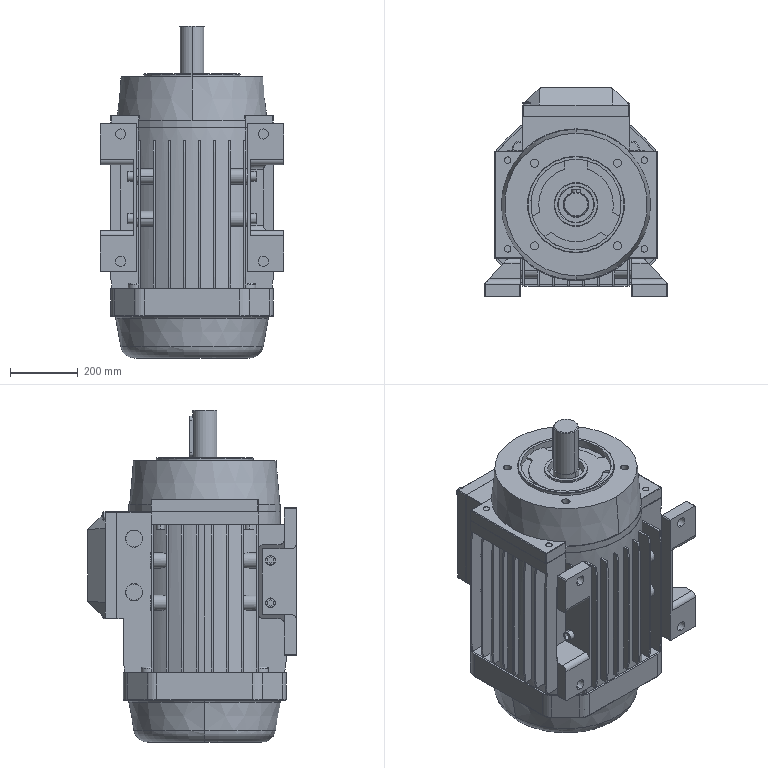Part | SolidWorks | features ICE 38, Fillet 18, MirrorPattern 10, Extrusion 5, CirPattern 4, Revolution 4, LibraryFeature 3, Chamfer 2, Dome 2, LPattern 2, CombineBodies 1, Scale 1, Shell 1 | 2 solids | 1459 faces | box 540 x 615 x 978 mm | volume 147963352 mm3 | plane 1138 | cylinder 237 | torus 58 | cone 16 | sphere 10 | commonest cylinder face diameters 30 x32 45 x32 3 x24 24 x20 6 x16 19.2 x16